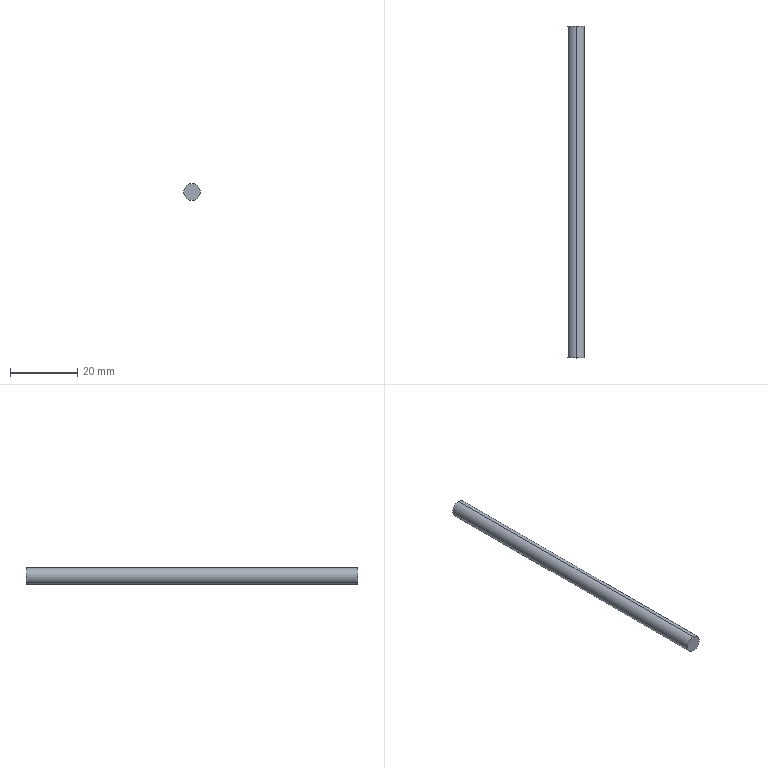Part | SolidWorks | features MBimport 1 | 1 solid | 4 faces | box 5 x 99 x 5 mm | volume 1944 mm3 | cylinder 2 | plane 2 | commonest cylinder face diameters 5 x2
STEP:
#1=CARTESIAN_POINT('',(0.,99.,2.5));
#2=VERTEX_POINT('',#1);
#3=CARTESIAN_POINT('',(0.,99.,-2.5));
#4=VERTEX_POINT('',#3);
#5=CARTESIAN_POINT('',(0.,99.,0.));
#6=DIRECTION('',(0.,1.,0.));
#7=DIRECTION('',(1.,0.,0.));
#8=AXIS2_PLACEMENT_3D('',#5,#6,#7);
#9=CIRCLE('',#8,2.5);
#10=EDGE_CURVE('',#2,#4,#9,.T.);
#11=ORIENTED_EDGE('',*,*,#10,.F.);
#12=CARTESIAN_POINT('',(0.,0.,2.5));
#13=VERTEX_POINT('',#12);
#14=CARTESIAN_POINT('',(0.,99.,2.5));
#15=DIRECTION('',(0.,-1.,0.));
#16=VECTOR('',#15,1000.);
#17=LINE('',#14,#16);
#18=EDGE_CURVE('',#2,#13,#17,.T.);
#19=ORIENTED_EDGE('',*,*,#18,.T.);
#20=CARTESIAN_POINT('',(0.,0.,-2.5));
#21=VERTEX_POINT('',#20);
#22=CARTESIAN_POINT('',(0.,0.,0.));
#23=DIRECTION('',(0.,1.,0.));
#24=DIRECTION('',(1.,0.,0.));
#25=AXIS2_PLACEMENT_3D('',#22,#23,#24);
#26=CIRCLE('',#25,2.5);
#27=EDGE_CURVE('',#13,#21,#26,.T.);
#28=ORIENTED_EDGE('',*,*,#27,.T.);
#29=CARTESIAN_POINT('',(0.,99.,-2.5));
#30=DIRECTION('',(0.,-1.,0.));
#31=VECTOR('',#30,1000.);
#32=LINE('',#29,#31);
#33=EDGE_CURVE('',#4,#21,#32,.T.);
#34=ORIENTED_EDGE('',*,*,#33,.F.);
#35=EDGE_LOOP('',(#11,#19,#28,#34));
#36=FACE_OUTER_BOUND('',#35,.T.);
#37=CARTESIAN_POINT('',(0.,99.,0.));
#38=DIRECTION('',(0.,-1.,0.));
#39=DIRECTION('',(0.,0.,-1.));
#40=AXIS2_PLACEMENT_3D('',#37,#38,#39);
#41=CYLINDRICAL_SURFACE('',#40,2.5);
#42=ADVANCED_FACE('',(#36),#41,.T.);
#43=ORIENTED_EDGE('',*,*,#18,.F.);
#44=CARTESIAN_POINT('',(0.,99.,0.));
#45=DIRECTION('',(0.,1.,0.));
#46=DIRECTION('',(1.,0.,0.));
#47=AXIS2_PLACEMENT_3D('',#44,#45,#46);
#48=CIRCLE('',#47,2.5);
#49=EDGE_CURVE('',#4,#2,#48,.T.);
#50=ORIENTED_EDGE('',*,*,#49,.F.);
#51=ORIENTED_EDGE('',*,*,#33,.T.);
#52=CARTESIAN_POINT('',(0.,0.,0.));
#53=DIRECTION('',(0.,1.,0.));
#54=DIRECTION('',(1.,0.,0.));
#55=AXIS2_PLACEMENT_3D('',#52,#53,#54);
#56=CIRCLE('',#55,2.5);
#57=EDGE_CURVE('',#21,#13,#56,.T.);
#58=ORIENTED_EDGE('',*,*,#57,.T.);
#59=EDGE_LOOP('',(#43,#50,#51,#58));
#60=FACE_OUTER_BOUND('',#59,.T.);
#61=CARTESIAN_POINT('',(0.,99.,0.));
#62=DIRECTION('',(0.,-1.,0.));
#63=DIRECTION('',(0.,0.,-1.));
#64=AXIS2_PLACEMENT_3D('',#61,#62,#63);
#65=CYLINDRICAL_SURFACE('',#64,2.5);
#66=ADVANCED_FACE('',(#60),#65,.T.);
#67=ORIENTED_EDGE('',*,*,#49,.T.);
#68=ORIENTED_EDGE('',*,*,#10,.T.);
#69=EDGE_LOOP('',(#67,#68));
#70=FACE_OUTER_BOUND('',#69,.T.);
#71=CARTESIAN_POINT('',(0.,99.,0.));
#72=DIRECTION('',(0.,1.,0.));
#73=DIRECTION('',(1.,0.,0.));
#74=AXIS2_PLACEMENT_3D('',#71,#72,#73);
#75=PLANE('',#74);
#76=ADVANCED_FACE('',(#70),#75,.T.);
#77=ORIENTED_EDGE('',*,*,#57,.F.);
#78=ORIENTED_EDGE('',*,*,#27,.F.);
#79=EDGE_LOOP('',(#77,#78));
#80=FACE_OUTER_BOUND('',#79,.T.);
#81=CARTESIAN_POINT('',(0.,0.,0.));
#82=DIRECTION('',(0.,1.,0.));
#83=DIRECTION('',(1.,0.,0.));
#84=AXIS2_PLACEMENT_3D('',#81,#82,#83);
#85=PLANE('',#84);
#86=ADVANCED_FACE('',(#80),#85,.F.);
#87=CLOSED_SHELL('',(#42,#66,#76,#86));
#88=MANIFOLD_SOLID_BREP('',#87);
#89=CARTESIAN_POINT('',(0.,0.,0.));
#90=DIRECTION('',(0.,0.,1.));
#91=DIRECTION('',(1.,0.,0.));
#92=AXIS2_PLACEMENT_3D('',#89,#90,#91);
#93=(LENGTH_UNIT()NAMED_UNIT(*)SI_UNIT(.MILLI.,.METRE.));
#94=UNCERTAINTY_MEASURE_WITH_UNIT(LENGTH_MEASURE(0.00001),#93,'','');
#95=(NAMED_UNIT(*)PLANE_ANGLE_UNIT()SI_UNIT($,.RADIAN.));
#96=(NAMED_UNIT(*)SI_UNIT($,.STERADIAN.)SOLID_ANGLE_UNIT());
#97=(GEOMETRIC_REPRESENTATION_CONTEXT(3)GLOBAL_UNCERTAINTY_ASSIGNED_CONTEXT((#94))GLOBAL_UNIT_ASSIGNED_CONTEXT((#93,#95,#96))REPRESENTATION_CONTEXT('',''));
#98=ADVANCED_BREP_SHAPE_REPRESENTATION('',(#88,#92),#97);